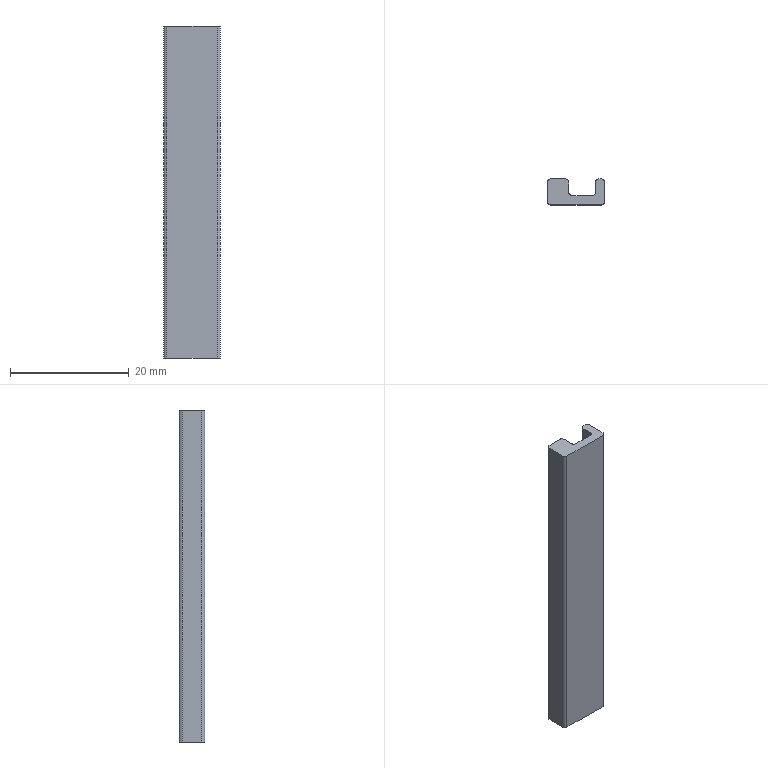Part | NX | features BREP 2 | 2 solids | 36 faces | box 9.6 x 4.3 x 56 mm | volume 3188 mm3 | plane 20 | cylinder 16 | commonest cylinder face diameters 1 x16
STEP:
#1=CARTESIAN_POINT('',(-4.3,2.15,-4.));
#2=VERTEX_POINT('',#1);
#3=CARTESIAN_POINT('',(-4.3,2.15,52.));
#4=VERTEX_POINT('',#3);
#5=CARTESIAN_POINT('',(-4.3,2.15,0.));
#6=DIRECTION('',(0.,0.,1.));
#7=VECTOR('',#6,1000.);
#8=LINE('',#5,#7);
#9=EDGE_CURVE('',#2,#4,#8,.T.);
#10=ORIENTED_EDGE('',*,*,#9,.T.);
#11=CARTESIAN_POINT('',(-1.7,2.15,52.));
#12=VERTEX_POINT('',#11);
#13=CARTESIAN_POINT('',(9.373,2.15,52.));
#14=DIRECTION('',(-1.,0.,0.));
#15=VECTOR('',#14,1000.);
#16=LINE('',#13,#15);
#17=EDGE_CURVE('',#12,#4,#16,.T.);
#18=ORIENTED_EDGE('',*,*,#17,.F.);
#19=CARTESIAN_POINT('',(-1.7,2.15,-4.));
#20=VERTEX_POINT('',#19);
#21=CARTESIAN_POINT('',(-1.7,2.15,0.));
#22=DIRECTION('',(0.,0.,1.));
#23=VECTOR('',#22,1000.);
#24=LINE('',#21,#23);
#25=EDGE_CURVE('',#20,#12,#24,.T.);
#26=ORIENTED_EDGE('',*,*,#25,.F.);
#27=CARTESIAN_POINT('',(9.373,2.15,-4.));
#28=DIRECTION('',(-1.,0.,0.));
#29=VECTOR('',#28,1000.);
#30=LINE('',#27,#29);
#31=EDGE_CURVE('',#20,#2,#30,.T.);
#32=ORIENTED_EDGE('',*,*,#31,.T.);
#33=EDGE_LOOP('',(#10,#18,#26,#32));
#34=FACE_BOUND('',#33,.T.);
#35=CARTESIAN_POINT('',(-1.7,2.15,0.));
#36=DIRECTION('',(0.,1.,0.));
#37=DIRECTION('',(1.,0.,0.));
#38=AXIS2_PLACEMENT_3D('',#35,#36,#37);
#39=PLANE('',#38);
#40=ADVANCED_FACE('',(#34),#39,.T.);
#41=ORIENTED_EDGE('',*,*,#25,.T.);
#42=CARTESIAN_POINT('',(-1.2,1.65,52.));
#43=VERTEX_POINT('',#42);
#44=CARTESIAN_POINT('',(-1.7,1.65,52.));
#45=DIRECTION('',(0.,0.,1.));
#46=DIRECTION('',(1.,0.,0.));
#47=AXIS2_PLACEMENT_3D('',#44,#45,#46);
#48=CIRCLE('',#47,0.5);
#49=EDGE_CURVE('',#43,#12,#48,.T.);
#50=ORIENTED_EDGE('',*,*,#49,.F.);
#51=CARTESIAN_POINT('',(-1.2,1.65,-4.));
#52=VERTEX_POINT('',#51);
#53=CARTESIAN_POINT('',(-1.2,1.65,0.));
#54=DIRECTION('',(0.,0.,1.));
#55=VECTOR('',#54,1000.);
#56=LINE('',#53,#55);
#57=EDGE_CURVE('',#52,#43,#56,.T.);
#58=ORIENTED_EDGE('',*,*,#57,.F.);
#59=CARTESIAN_POINT('',(-1.7,1.65,-4.));
#60=DIRECTION('',(0.,0.,1.));
#61=DIRECTION('',(1.,0.,0.));
#62=AXIS2_PLACEMENT_3D('',#59,#60,#61);
#63=CIRCLE('',#62,0.5);
#64=EDGE_CURVE('',#52,#20,#63,.T.);
#65=ORIENTED_EDGE('',*,*,#64,.T.);
#66=EDGE_LOOP('',(#41,#50,#58,#65));
#67=FACE_BOUND('',#66,.T.);
#68=CARTESIAN_POINT('',(-1.7,1.65,0.));
#69=DIRECTION('',(0.,0.,1.));
#70=DIRECTION('',(-1.,0.,0.));
#71=AXIS2_PLACEMENT_3D('',#68,#69,#70);
#72=CYLINDRICAL_SURFACE('',#71,0.5);
#73=ADVANCED_FACE('',(#67),#72,.T.);
#74=ORIENTED_EDGE('',*,*,#57,.T.);
#75=CARTESIAN_POINT('',(-1.2,-0.15,52.));
#76=VERTEX_POINT('',#75);
#77=CARTESIAN_POINT('',(-1.2,1.628,52.));
#78=DIRECTION('',(0.,1.,0.));
#79=VECTOR('',#78,1000.);
#80=LINE('',#77,#79);
#81=EDGE_CURVE('',#76,#43,#80,.T.);
#82=ORIENTED_EDGE('',*,*,#81,.F.);
#83=CARTESIAN_POINT('',(-1.2,-0.15,-4.));
#84=VERTEX_POINT('',#83);
#85=CARTESIAN_POINT('',(-1.2,-0.15,0.));
#86=DIRECTION('',(0.,0.,1.));
#87=VECTOR('',#86,1000.);
#88=LINE('',#85,#87);
#89=EDGE_CURVE('',#84,#76,#88,.T.);
#90=ORIENTED_EDGE('',*,*,#89,.F.);
#91=CARTESIAN_POINT('',(-1.2,1.628,-4.));
#92=DIRECTION('',(0.,1.,0.));
#93=VECTOR('',#92,1000.);
#94=LINE('',#91,#93);
#95=EDGE_CURVE('',#84,#52,#94,.T.);
#96=ORIENTED_EDGE('',*,*,#95,.T.);
#97=EDGE_LOOP('',(#74,#82,#90,#96));
#98=FACE_BOUND('',#97,.T.);
#99=CARTESIAN_POINT('',(-1.2,-0.15,0.));
#100=DIRECTION('',(1.,0.,0.));
#101=DIRECTION('',(0.,-1.,0.));
#102=AXIS2_PLACEMENT_3D('',#99,#100,#101);
#103=PLANE('',#102);
#104=ADVANCED_FACE('',(#98),#103,.T.);
#105=ORIENTED_EDGE('',*,*,#89,.T.);
#106=CARTESIAN_POINT('',(-0.7,-0.65,52.));
#107=VERTEX_POINT('',#106);
#108=CARTESIAN_POINT('',(-0.7,-0.15,52.));
#109=DIRECTION('',(0.,0.,-1.));
#110=DIRECTION('',(1.,0.,0.));
#111=AXIS2_PLACEMENT_3D('',#108,#109,#110);
#112=CIRCLE('',#111,0.5);
#113=EDGE_CURVE('',#107,#76,#112,.T.);
#114=ORIENTED_EDGE('',*,*,#113,.F.);
#115=CARTESIAN_POINT('',(-0.7,-0.65,-4.));
#116=VERTEX_POINT('',#115);
#117=CARTESIAN_POINT('',(-0.7,-0.65,0.));
#118=DIRECTION('',(0.,0.,1.));
#119=VECTOR('',#118,1000.);
#120=LINE('',#117,#119);
#121=EDGE_CURVE('',#116,#107,#120,.T.);
#122=ORIENTED_EDGE('',*,*,#121,.F.);
#123=CARTESIAN_POINT('',(-0.7,-0.15,-4.));
#124=DIRECTION('',(0.,0.,-1.));
#125=DIRECTION('',(1.,0.,0.));
#126=AXIS2_PLACEMENT_3D('',#123,#124,#125);
#127=CIRCLE('',#126,0.5);
#128=EDGE_CURVE('',#116,#84,#127,.T.);
#129=ORIENTED_EDGE('',*,*,#128,.T.);
#130=EDGE_LOOP('',(#105,#114,#122,#129));
#131=FACE_BOUND('',#130,.T.);
#132=CARTESIAN_POINT('',(-0.7,-0.15,0.));
#133=DIRECTION('',(0.,0.,1.));
#134=DIRECTION('',(-1.,0.,0.));
#135=AXIS2_PLACEMENT_3D('',#132,#133,#134);
#136=CYLINDRICAL_SURFACE('',#135,0.5);
#137=ADVANCED_FACE('',(#131),#136,.F.);
#138=ORIENTED_EDGE('',*,*,#121,.T.);
#139=CARTESIAN_POINT('',(2.8,-0.65,52.));
#140=VERTEX_POINT('',#139);
#141=CARTESIAN_POINT('',(9.373,-0.65,52.));
#142=DIRECTION('',(-1.,0.,0.));
#143=VECTOR('',#142,1000.);
#144=LINE('',#141,#143);
#145=EDGE_CURVE('',#140,#107,#144,.T.);
#146=ORIENTED_EDGE('',*,*,#145,.F.);
#147=CARTESIAN_POINT('',(2.8,-0.65,-4.));
#148=VERTEX_POINT('',#147);
#149=CARTESIAN_POINT('',(2.8,-0.65,0.));
#150=DIRECTION('',(0.,0.,1.));
#151=VECTOR('',#150,1000.);
#152=LINE('',#149,#151);
#153=EDGE_CURVE('',#148,#140,#152,.T.);
#154=ORIENTED_EDGE('',*,*,#153,.F.);
#155=CARTESIAN_POINT('',(9.373,-0.65,-4.));
#156=DIRECTION('',(-1.,0.,0.));
#157=VECTOR('',#156,1000.);
#158=LINE('',#155,#157);
#159=EDGE_CURVE('',#148,#116,#158,.T.);
#160=ORIENTED_EDGE('',*,*,#159,.T.);
#161=EDGE_LOOP('',(#138,#146,#154,#160));
#162=FACE_BOUND('',#161,.T.);
#163=CARTESIAN_POINT('',(2.8,-0.65,0.));
#164=DIRECTION('',(0.,1.,0.));
#165=DIRECTION('',(1.,0.,0.));
#166=AXIS2_PLACEMENT_3D('',#163,#164,#165);
#167=PLANE('',#166);
#168=ADVANCED_FACE('',(#162),#167,.T.);
#169=ORIENTED_EDGE('',*,*,#153,.T.);
#170=CARTESIAN_POINT('',(3.3,-0.15,52.));
#171=VERTEX_POINT('',#170);
#172=CARTESIAN_POINT('',(2.8,-0.15,52.));
#173=DIRECTION('',(0.,0.,-1.));
#174=DIRECTION('',(1.,0.,0.));
#175=AXIS2_PLACEMENT_3D('',#172,#173,#174);
#176=CIRCLE('',#175,0.5);
#177=EDGE_CURVE('',#171,#140,#176,.T.);
#178=ORIENTED_EDGE('',*,*,#177,.F.);
#179=CARTESIAN_POINT('',(3.3,-0.15,-4.));
#180=VERTEX_POINT('',#179);
#181=CARTESIAN_POINT('',(3.3,-0.15,0.));
#182=DIRECTION('',(0.,0.,1.));
#183=VECTOR('',#182,1000.);
#184=LINE('',#181,#183);
#185=EDGE_CURVE('',#180,#171,#184,.T.);
#186=ORIENTED_EDGE('',*,*,#185,.F.);
#187=CARTESIAN_POINT('',(2.8,-0.15,-4.));
#188=DIRECTION('',(0.,0.,-1.));
#189=DIRECTION('',(1.,0.,0.));
#190=AXIS2_PLACEMENT_3D('',#187,#188,#189);
#191=CIRCLE('',#190,0.5);
#192=EDGE_CURVE('',#180,#148,#191,.T.);
#193=ORIENTED_EDGE('',*,*,#192,.T.);
#194=EDGE_LOOP('',(#169,#178,#186,#193));
#195=FACE_BOUND('',#194,.T.);
#196=CARTESIAN_POINT('',(2.8,-0.15,0.));
#197=DIRECTION('',(0.,0.,1.));
#198=DIRECTION('',(-1.,0.,0.));
#199=AXIS2_PLACEMENT_3D('',#196,#197,#198);
#200=CYLINDRICAL_SURFACE('',#199,0.5);
#201=ADVANCED_FACE('',(#195),#200,.F.);
#202=ORIENTED_EDGE('',*,*,#185,.T.);
#203=CARTESIAN_POINT('',(3.3,1.65,52.));
#204=VERTEX_POINT('',#203);
#205=CARTESIAN_POINT('',(3.3,1.628,52.));
#206=DIRECTION('',(0.,-1.,0.));
#207=VECTOR('',#206,1000.);
#208=LINE('',#205,#207);
#209=EDGE_CURVE('',#204,#171,#208,.T.);
#210=ORIENTED_EDGE('',*,*,#209,.F.);
#211=CARTESIAN_POINT('',(3.3,1.65,-4.));
#212=VERTEX_POINT('',#211);
#213=CARTESIAN_POINT('',(3.3,1.65,0.));
#214=DIRECTION('',(0.,0.,1.));
#215=VECTOR('',#214,1000.);
#216=LINE('',#213,#215);
#217=EDGE_CURVE('',#212,#204,#216,.T.);
#218=ORIENTED_EDGE('',*,*,#217,.F.);
#219=CARTESIAN_POINT('',(3.3,1.628,-4.));
#220=DIRECTION('',(0.,-1.,0.));
#221=VECTOR('',#220,1000.);
#222=LINE('',#219,#221);
#223=EDGE_CURVE('',#212,#180,#222,.T.);
#224=ORIENTED_EDGE('',*,*,#223,.T.);
#225=EDGE_LOOP('',(#202,#210,#218,#224));
#226=FACE_BOUND('',#225,.T.);
#227=CARTESIAN_POINT('',(3.3,1.65,0.));
#228=DIRECTION('',(-1.,0.,0.));
#229=DIRECTION('',(0.,1.,0.));
#230=AXIS2_PLACEMENT_3D('',#227,#228,#229);
#231=PLANE('',#230);
#232=ADVANCED_FACE('',(#226),#231,.T.);
#233=ORIENTED_EDGE('',*,*,#217,.T.);
#234=CARTESIAN_POINT('',(3.8,2.15,52.));
#235=VERTEX_POINT('',#234);
#236=CARTESIAN_POINT('',(3.8,1.65,52.));
#237=DIRECTION('',(0.,0.,1.));
#238=DIRECTION('',(1.,0.,0.));
#239=AXIS2_PLACEMENT_3D('',#236,#237,#238);
#240=CIRCLE('',#239,0.5);
#241=EDGE_CURVE('',#235,#204,#240,.T.);
#242=ORIENTED_EDGE('',*,*,#241,.F.);
#243=CARTESIAN_POINT('',(3.8,2.15,-4.));
#244=VERTEX_POINT('',#243);
#245=CARTESIAN_POINT('',(3.8,2.15,0.));
#246=DIRECTION('',(0.,0.,1.));
#247=VECTOR('',#246,1000.);
#248=LINE('',#245,#247);
#249=EDGE_CURVE('',#244,#235,#248,.T.);
#250=ORIENTED_EDGE('',*,*,#249,.F.);
#251=CARTESIAN_POINT('',(3.8,1.65,-4.));
#252=DIRECTION('',(0.,0.,1.));
#253=DIRECTION('',(1.,0.,0.));
#254=AXIS2_PLACEMENT_3D('',#251,#252,#253);
#255=CIRCLE('',#254,0.5);
#256=EDGE_CURVE('',#244,#212,#255,.T.);
#257=ORIENTED_EDGE('',*,*,#256,.T.);
#258=EDGE_LOOP('',(#233,#242,#250,#257));
#259=FACE_BOUND('',#258,.T.);
#260=CARTESIAN_POINT('',(3.8,1.65,0.));
#261=DIRECTION('',(0.,0.,1.));
#262=DIRECTION('',(-1.,0.,0.));
#263=AXIS2_PLACEMENT_3D('',#260,#261,#262);
#264=CYLINDRICAL_SURFACE('',#263,0.5);
#265=ADVANCED_FACE('',(#259),#264,.T.);
#266=ORIENTED_EDGE('',*,*,#249,.T.);
#267=CARTESIAN_POINT('',(4.3,2.15,52.));
#268=VERTEX_POINT('',#267);
#269=CARTESIAN_POINT('',(9.373,2.15,52.));
#270=DIRECTION('',(-1.,0.,0.));
#271=VECTOR('',#270,1000.);
#272=LINE('',#269,#271);
#273=EDGE_CURVE('',#268,#235,#272,.T.);
#274=ORIENTED_EDGE('',*,*,#273,.F.);
#275=CARTESIAN_POINT('',(4.3,2.15,-4.));
#276=VERTEX_POINT('',#275);
#277=CARTESIAN_POINT('',(4.3,2.15,0.));
#278=DIRECTION('',(0.,0.,1.));
#279=VECTOR('',#278,1000.);
#280=LINE('',#277,#279);
#281=EDGE_CURVE('',#276,#268,#280,.T.);
#282=ORIENTED_EDGE('',*,*,#281,.F.);
#283=CARTESIAN_POINT('',(9.373,2.15,-4.));
#284=DIRECTION('',(-1.,0.,0.));
#285=VECTOR('',#284,1000.);
#286=LINE('',#283,#285);
#287=EDGE_CURVE('',#276,#244,#286,.T.);
#288=ORIENTED_EDGE('',*,*,#287,.T.);
#289=EDGE_LOOP('',(#266,#274,#282,#288));
#290=FACE_BOUND('',#289,.T.);
#291=CARTESIAN_POINT('',(4.3,2.15,0.));
#292=DIRECTION('',(0.,1.,0.));
#293=DIRECTION('',(1.,0.,0.));
#294=AXIS2_PLACEMENT_3D('',#291,#292,#293);
#295=PLANE('',#294);
#296=ADVANCED_FACE('',(#290),#295,.T.);
#297=ORIENTED_EDGE('',*,*,#281,.T.);
#298=CARTESIAN_POINT('',(4.8,1.65,52.));
#299=VERTEX_POINT('',#298);
#300=CARTESIAN_POINT('',(4.3,1.65,52.));
#301=DIRECTION('',(0.,0.,1.));
#302=DIRECTION('',(1.,0.,0.));
#303=AXIS2_PLACEMENT_3D('',#300,#301,#302);
#304=CIRCLE('',#303,0.5);
#305=EDGE_CURVE('',#299,#268,#304,.T.);
#306=ORIENTED_EDGE('',*,*,#305,.F.);
#307=CARTESIAN_POINT('',(4.8,1.65,-4.));
#308=VERTEX_POINT('',#307);
#309=CARTESIAN_POINT('',(4.8,1.65,0.));
#310=DIRECTION('',(0.,0.,1.));
#311=VECTOR('',#310,1000.);
#312=LINE('',#309,#311);
#313=EDGE_CURVE('',#308,#299,#312,.T.);
#314=ORIENTED_EDGE('',*,*,#313,.F.);
#315=CARTESIAN_POINT('',(4.3,1.65,-4.));
#316=DIRECTION('',(0.,0.,1.));
#317=DIRECTION('',(1.,0.,0.));
#318=AXIS2_PLACEMENT_3D('',#315,#316,#317);
#319=CIRCLE('',#318,0.5);
#320=EDGE_CURVE('',#308,#276,#319,.T.);
#321=ORIENTED_EDGE('',*,*,#320,.T.);
#322=EDGE_LOOP('',(#297,#306,#314,#321));
#323=FACE_BOUND('',#322,.T.);
#324=CARTESIAN_POINT('',(4.3,1.65,0.));
#325=DIRECTION('',(0.,0.,1.));
#326=DIRECTION('',(-1.,0.,0.));
#327=AXIS2_PLACEMENT_3D('',#324,#325,#326);
#328=CYLINDRICAL_SURFACE('',#327,0.5);
#329=ADVANCED_FACE('',(#323),#328,.T.);
#330=ORIENTED_EDGE('',*,*,#313,.T.);
#331=CARTESIAN_POINT('',(4.8,-1.65,52.));
#332=VERTEX_POINT('',#331);
#333=CARTESIAN_POINT('',(4.8,1.628,52.));
#334=DIRECTION('',(0.,1.,0.));
#335=VECTOR('',#334,1000.);
#336=LINE('',#333,#335);
#337=EDGE_CURVE('',#332,#299,#336,.T.);
#338=ORIENTED_EDGE('',*,*,#337,.F.);
#339=CARTESIAN_POINT('',(4.8,-1.65,-4.));
#340=VERTEX_POINT('',#339);
#341=CARTESIAN_POINT('',(4.8,-1.65,0.));
#342=DIRECTION('',(0.,0.,1.));
#343=VECTOR('',#342,1000.);
#344=LINE('',#341,#343);
#345=EDGE_CURVE('',#340,#332,#344,.T.);
#346=ORIENTED_EDGE('',*,*,#345,.F.);
#347=CARTESIAN_POINT('',(4.8,1.628,-4.));
#348=DIRECTION('',(0.,1.,0.));
#349=VECTOR('',#348,1000.);
#350=LINE('',#347,#349);
#351=EDGE_CURVE('',#340,#308,#350,.T.);
#352=ORIENTED_EDGE('',*,*,#351,.T.);
#353=EDGE_LOOP('',(#330,#338,#346,#352));
#354=FACE_BOUND('',#353,.T.);
#355=CARTESIAN_POINT('',(4.8,-1.65,0.));
#356=DIRECTION('',(1.,0.,0.));
#357=DIRECTION('',(0.,-1.,0.));
#358=AXIS2_PLACEMENT_3D('',#355,#356,#357);
#359=PLANE('',#358);
#360=ADVANCED_FACE('',(#354),#359,.T.);
#361=ORIENTED_EDGE('',*,*,#345,.T.);
#362=CARTESIAN_POINT('',(4.3,-2.15,52.));
#363=VERTEX_POINT('',#362);
#364=CARTESIAN_POINT('',(4.3,-1.65,52.));
#365=DIRECTION('',(0.,0.,1.));
#366=DIRECTION('',(1.,0.,0.));
#367=AXIS2_PLACEMENT_3D('',#364,#365,#366);
#368=CIRCLE('',#367,0.5);
#369=EDGE_CURVE('',#363,#332,#368,.T.);
#370=ORIENTED_EDGE('',*,*,#369,.F.);
#371=CARTESIAN_POINT('',(4.3,-2.15,-4.));
#372=VERTEX_POINT('',#371);
#373=CARTESIAN_POINT('',(4.3,-2.15,0.));
#374=DIRECTION('',(0.,0.,1.));
#375=VECTOR('',#374,1000.);
#376=LINE('',#373,#375);
#377=EDGE_CURVE('',#372,#363,#376,.T.);
#378=ORIENTED_EDGE('',*,*,#377,.F.);
#379=CARTESIAN_POINT('',(4.3,-1.65,-4.));
#380=DIRECTION('',(0.,0.,1.));
#381=DIRECTION('',(1.,0.,0.));
#382=AXIS2_PLACEMENT_3D('',#379,#380,#381);
#383=CIRCLE('',#382,0.5);
#384=EDGE_CURVE('',#372,#340,#383,.T.);
#385=ORIENTED_EDGE('',*,*,#384,.T.);
#386=EDGE_LOOP('',(#361,#370,#378,#385));
#387=FACE_BOUND('',#386,.T.);
#388=CARTESIAN_POINT('',(4.3,-1.65,0.));
#389=DIRECTION('',(0.,0.,1.));
#390=DIRECTION('',(-1.,0.,0.));
#391=AXIS2_PLACEMENT_3D('',#388,#389,#390);
#392=CYLINDRICAL_SURFACE('',#391,0.5);
#393=ADVANCED_FACE('',(#387),#392,.T.);
#394=ORIENTED_EDGE('',*,*,#377,.T.);
#395=CARTESIAN_POINT('',(-4.3,-2.15,52.));
#396=VERTEX_POINT('',#395);
#397=CARTESIAN_POINT('',(9.373,-2.15,52.));
#398=DIRECTION('',(1.,0.,0.));
#399=VECTOR('',#398,1000.);
#400=LINE('',#397,#399);
#401=EDGE_CURVE('',#396,#363,#400,.T.);
#402=ORIENTED_EDGE('',*,*,#401,.F.);
#403=CARTESIAN_POINT('',(-4.3,-2.15,-4.));
#404=VERTEX_POINT('',#403);
#405=CARTESIAN_POINT('',(-4.3,-2.15,0.));
#406=DIRECTION('',(0.,0.,1.));
#407=VECTOR('',#406,1000.);
#408=LINE('',#405,#407);
#409=EDGE_CURVE('',#404,#396,#408,.T.);
#410=ORIENTED_EDGE('',*,*,#409,.F.);
#411=CARTESIAN_POINT('',(9.373,-2.15,-4.));
#412=DIRECTION('',(1.,0.,0.));
#413=VECTOR('',#412,1000.);
#414=LINE('',#411,#413);
#415=EDGE_CURVE('',#404,#372,#414,.T.);
#416=ORIENTED_EDGE('',*,*,#415,.T.);
#417=EDGE_LOOP('',(#394,#402,#410,#416));
#418=FACE_BOUND('',#417,.T.);
#419=CARTESIAN_POINT('',(-4.3,-2.15,0.));
#420=DIRECTION('',(0.,-1.,0.));
#421=DIRECTION('',(-1.,0.,0.));
#422=AXIS2_PLACEMENT_3D('',#419,#420,#421);
#423=PLANE('',#422);
#424=ADVANCED_FACE('',(#418),#423,.T.);
#425=ORIENTED_EDGE('',*,*,#409,.T.);
#426=CARTESIAN_POINT('',(-4.8,-1.65,52.));
#427=VERTEX_POINT('',#426);
#428=CARTESIAN_POINT('',(-4.3,-1.65,52.));
#429=DIRECTION('',(0.,0.,1.));
#430=DIRECTION('',(1.,0.,0.));
#431=AXIS2_PLACEMENT_3D('',#428,#429,#430);
#432=CIRCLE('',#431,0.5);
#433=EDGE_CURVE('',#427,#396,#432,.T.);
#434=ORIENTED_EDGE('',*,*,#433,.F.);
#435=CARTESIAN_POINT('',(-4.8,-1.65,-4.));
#436=VERTEX_POINT('',#435);
#437=CARTESIAN_POINT('',(-4.8,-1.65,0.));
#438=DIRECTION('',(0.,0.,1.));
#439=VECTOR('',#438,1000.);
#440=LINE('',#437,#439);
#441=EDGE_CURVE('',#436,#427,#440,.T.);
#442=ORIENTED_EDGE('',*,*,#441,.F.);
#443=CARTESIAN_POINT('',(-4.3,-1.65,-4.));
#444=DIRECTION('',(0.,0.,1.));
#445=DIRECTION('',(1.,0.,0.));
#446=AXIS2_PLACEMENT_3D('',#443,#444,#445);
#447=CIRCLE('',#446,0.5);
#448=EDGE_CURVE('',#436,#404,#447,.T.);
#449=ORIENTED_EDGE('',*,*,#448,.T.);
#450=EDGE_LOOP('',(#425,#434,#442,#449));
#451=FACE_BOUND('',#450,.T.);
#452=CARTESIAN_POINT('',(-4.3,-1.65,0.));
#453=DIRECTION('',(0.,0.,1.));
#454=DIRECTION('',(-1.,0.,0.));
#455=AXIS2_PLACEMENT_3D('',#452,#453,#454);
#456=CYLINDRICAL_SURFACE('',#455,0.5);
#457=ADVANCED_FACE('',(#451),#456,.T.);
#458=ORIENTED_EDGE('',*,*,#441,.T.);
#459=CARTESIAN_POINT('',(-4.8,1.65,52.));
#460=VERTEX_POINT('',#459);
#461=CARTESIAN_POINT('',(-4.8,1.628,52.));
#462=DIRECTION('',(0.,-1.,0.));
#463=VECTOR('',#462,1000.);
#464=LINE('',#461,#463);
#465=EDGE_CURVE('',#460,#427,#464,.T.);
#466=ORIENTED_EDGE('',*,*,#465,.F.);
#467=CARTESIAN_POINT('',(-4.8,1.65,-4.));
#468=VERTEX_POINT('',#467);
#469=CARTESIAN_POINT('',(-4.8,1.65,0.));
#470=DIRECTION('',(0.,0.,1.));
#471=VECTOR('',#470,1000.);
#472=LINE('',#469,#471);
#473=EDGE_CURVE('',#468,#460,#472,.T.);
#474=ORIENTED_EDGE('',*,*,#473,.F.);
#475=CARTESIAN_POINT('',(-4.8,1.628,-4.));
#476=DIRECTION('',(0.,-1.,0.));
#477=VECTOR('',#476,1000.);
#478=LINE('',#475,#477);
#479=EDGE_CURVE('',#468,#436,#478,.T.);
#480=ORIENTED_EDGE('',*,*,#479,.T.);
#481=EDGE_LOOP('',(#458,#466,#474,#480));
#482=FACE_BOUND('',#481,.T.);
#483=CARTESIAN_POINT('',(-4.8,1.65,0.));
#484=DIRECTION('',(-1.,0.,0.));
#485=DIRECTION('',(0.,1.,0.));
#486=AXIS2_PLACEMENT_3D('',#483,#484,#485);
#487=PLANE('',#486);
#488=ADVANCED_FACE('',(#482),#487,.T.);
#489=CARTESIAN_POINT('',(-4.3,1.65,-4.));
#490=DIRECTION('',(0.,0.,1.));
#491=DIRECTION('',(1.,0.,0.));
#492=AXIS2_PLACEMENT_3D('',#489,#490,#491);
#493=CIRCLE('',#492,0.5);
#494=EDGE_CURVE('',#2,#468,#493,.T.);
#495=ORIENTED_EDGE('',*,*,#494,.T.);
#496=ORIENTED_EDGE('',*,*,#473,.T.);
#497=CARTESIAN_POINT('',(-4.3,1.65,52.));
#498=DIRECTION('',(0.,0.,1.));
#499=DIRECTION('',(1.,0.,0.));
#500=AXIS2_PLACEMENT_3D('',#497,#498,#499);
#501=CIRCLE('',#500,0.5);
#502=EDGE_CURVE('',#4,#460,#501,.T.);
#503=ORIENTED_EDGE('',*,*,#502,.F.);
#504=ORIENTED_EDGE('',*,*,#9,.F.);
#505=EDGE_LOOP('',(#495,#496,#503,#504));
#506=FACE_BOUND('',#505,.T.);
#507=CARTESIAN_POINT('',(-4.3,1.65,0.));
#508=DIRECTION('',(0.,0.,1.));
#509=DIRECTION('',(-1.,0.,0.));
#510=AXIS2_PLACEMENT_3D('',#507,#508,#509);
#511=CYLINDRICAL_SURFACE('',#510,0.5);
#512=ADVANCED_FACE('',(#506),#511,.T.);
#513=ORIENTED_EDGE('',*,*,#465,.T.);
#514=ORIENTED_EDGE('',*,*,#433,.T.);
#515=ORIENTED_EDGE('',*,*,#401,.T.);
#516=ORIENTED_EDGE('',*,*,#369,.T.);
#517=ORIENTED_EDGE('',*,*,#337,.T.);
#518=ORIENTED_EDGE('',*,*,#305,.T.);
#519=ORIENTED_EDGE('',*,*,#273,.T.);
#520=ORIENTED_EDGE('',*,*,#241,.T.);
#521=ORIENTED_EDGE('',*,*,#209,.T.);
#522=ORIENTED_EDGE('',*,*,#177,.T.);
#523=ORIENTED_EDGE('',*,*,#145,.T.);
#524=ORIENTED_EDGE('',*,*,#113,.T.);
#525=ORIENTED_EDGE('',*,*,#81,.T.);
#526=ORIENTED_EDGE('',*,*,#49,.T.);
#527=ORIENTED_EDGE('',*,*,#17,.T.);
#528=ORIENTED_EDGE('',*,*,#502,.T.);
#529=EDGE_LOOP('',(#513,#514,#515,#516,#517,#518,#519,#520,#521,#522,#523,#524,#525,#526,#527,#528));
#530=FACE_BOUND('',#529,.T.);
#531=CARTESIAN_POINT('',(9.373,1.628,52.));
#532=DIRECTION('',(0.,0.,1.));
#533=DIRECTION('',(-1.,0.,0.));
#534=AXIS2_PLACEMENT_3D('',#531,#532,#533);
#535=PLANE('',#534);
#536=ADVANCED_FACE('',(#530),#535,.T.);
#537=ORIENTED_EDGE('',*,*,#479,.F.);
#538=ORIENTED_EDGE('',*,*,#494,.F.);
#539=ORIENTED_EDGE('',*,*,#31,.F.);
#540=ORIENTED_EDGE('',*,*,#64,.F.);
#541=ORIENTED_EDGE('',*,*,#95,.F.);
#542=ORIENTED_EDGE('',*,*,#128,.F.);
#543=ORIENTED_EDGE('',*,*,#159,.F.);
#544=ORIENTED_EDGE('',*,*,#192,.F.);
#545=ORIENTED_EDGE('',*,*,#223,.F.);
#546=ORIENTED_EDGE('',*,*,#256,.F.);
#547=ORIENTED_EDGE('',*,*,#287,.F.);
#548=ORIENTED_EDGE('',*,*,#320,.F.);
#549=ORIENTED_EDGE('',*,*,#351,.F.);
#550=ORIENTED_EDGE('',*,*,#384,.F.);
#551=ORIENTED_EDGE('',*,*,#415,.F.);
#552=ORIENTED_EDGE('',*,*,#448,.F.);
#553=EDGE_LOOP('',(#537,#538,#539,#540,#541,#542,#543,#544,#545,#546,#547,#548,#549,#550,#551,#552));
#554=FACE_BOUND('',#553,.T.);
#555=CARTESIAN_POINT('',(9.373,1.628,-4.));
#556=DIRECTION('',(0.,0.,1.));
#557=DIRECTION('',(-1.,0.,0.));
#558=AXIS2_PLACEMENT_3D('',#555,#556,#557);
#559=PLANE('',#558);
#560=ADVANCED_FACE('',(#554),#559,.F.);
#561=CLOSED_SHELL('',(#40,#73,#104,#137,#168,#201,#232,#265,#296,#329,#360,#393,#424,#457,#488,#512,#536,#560));
#562=MANIFOLD_SOLID_BREP('',#561);
#563=CARTESIAN_POINT('',(-4.3,2.15,-4.));
#564=VERTEX_POINT('',#563);
#565=CARTESIAN_POINT('',(-4.3,2.15,52.));
#566=VERTEX_POINT('',#565);
#567=CARTESIAN_POINT('',(-4.3,2.15,0.));
#568=DIRECTION('',(0.,0.,1.));
#569=VECTOR('',#568,1000.);
#570=LINE('',#567,#569);
#571=EDGE_CURVE('',#564,#566,#570,.T.);
#572=ORIENTED_EDGE('',*,*,#571,.T.);
#573=CARTESIAN_POINT('',(-1.7,2.15,52.));
#574=VERTEX_POINT('',#573);
#575=CARTESIAN_POINT('',(9.373,2.15,52.));
#576=DIRECTION('',(-1.,0.,0.));
#577=VECTOR('',#576,1000.);
#578=LINE('',#575,#577);
#579=EDGE_CURVE('',#574,#566,#578,.T.);
#580=ORIENTED_EDGE('',*,*,#579,.F.);
#581=CARTESIAN_POINT('',(-1.7,2.15,-4.));
#582=VERTEX_POINT('',#581);
#583=CARTESIAN_POINT('',(-1.7,2.15,0.));
#584=DIRECTION('',(0.,0.,1.));
#585=VECTOR('',#584,1000.);
#586=LINE('',#583,#585);
#587=EDGE_CURVE('',#582,#574,#586,.T.);
#588=ORIENTED_EDGE('',*,*,#587,.F.);
#589=CARTESIAN_POINT('',(9.373,2.15,-4.));
#590=DIRECTION('',(-1.,0.,0.));
#591=VECTOR('',#590,1000.);
#592=LINE('',#589,#591);
#593=EDGE_CURVE('',#582,#564,#592,.T.);
#594=ORIENTED_EDGE('',*,*,#593,.T.);
#595=EDGE_LOOP('',(#572,#580,#588,#594));
#596=FACE_BOUND('',#595,.T.);
#597=CARTESIAN_POINT('',(-1.7,2.15,0.));
#598=DIRECTION('',(0.,1.,0.));
#599=DIRECTION('',(1.,0.,0.));
#600=AXIS2_PLACEMENT_3D('',#597,#598,#599);
#601=PLANE('',#600);
#602=ADVANCED_FACE('',(#596),#601,.T.);
#603=ORIENTED_EDGE('',*,*,#587,.T.);
#604=CARTESIAN_POINT('',(-1.2,1.65,52.));
#605=VERTEX_POINT('',#604);
#606=CARTESIAN_POINT('',(-1.7,1.65,52.));
#607=DIRECTION('',(0.,0.,1.));
#608=DIRECTION('',(1.,0.,0.));
#609=AXIS2_PLACEMENT_3D('',#606,#607,#608);
#610=CIRCLE('',#609,0.5);
#611=EDGE_CURVE('',#605,#574,#610,.T.);
#612=ORIENTED_EDGE('',*,*,#611,.F.);
#613=CARTESIAN_POINT('',(-1.2,1.65,-4.));
#614=VERTEX_POINT('',#613);
#615=CARTESIAN_POINT('',(-1.2,1.65,0.));
#616=DIRECTION('',(0.,0.,1.));
#617=VECTOR('',#616,1000.);
#618=LINE('',#615,#617);
#619=EDGE_CURVE('',#614,#605,#618,.T.);
#620=ORIENTED_EDGE('',*,*,#619,.F.);
#621=CARTESIAN_POINT('',(-1.7,1.65,-4.));
#622=DIRECTION('',(0.,0.,1.));
#623=DIRECTION('',(1.,0.,0.));
#624=AXIS2_PLACEMENT_3D('',#621,#622,#623);
#625=CIRCLE('',#624,0.5);
#626=EDGE_CURVE('',#614,#582,#625,.T.);
#627=ORIENTED_EDGE('',*,*,#626,.T.);
#628=EDGE_LOOP('',(#603,#612,#620,#627));
#629=FACE_BOUND('',#628,.T.);
#630=CARTESIAN_POINT('',(-1.7,1.65,0.));
#631=DIRECTION('',(0.,0.,1.));
#632=DIRECTION('',(-1.,0.,0.));
#633=AXIS2_PLACEMENT_3D('',#630,#631,#632);
#634=CYLINDRICAL_SURFACE('',#633,0.5);
#635=ADVANCED_FACE('',(#629),#634,.T.);
#636=ORIENTED_EDGE('',*,*,#619,.T.);
#637=CARTESIAN_POINT('',(-1.2,-0.15,52.));
#638=VERTEX_POINT('',#637);
#639=CARTESIAN_POINT('',(-1.2,1.628,52.));
#640=DIRECTION('',(0.,1.,0.));
#641=VECTOR('',#640,1000.);
#642=LINE('',#639,#641);
#643=EDGE_CURVE('',#638,#605,#642,.T.);
#644=ORIENTED_EDGE('',*,*,#643,.F.);
#645=CARTESIAN_POINT('',(-1.2,-0.15,-4.));
#646=VERTEX_POINT('',#645);
#647=CARTESIAN_POINT('',(-1.2,-0.15,0.));
#648=DIRECTION('',(0.,0.,1.));
#649=VECTOR('',#648,1000.);
#650=LINE('',#647,#649);
#651=EDGE_CURVE('',#646,#638,#650,.T.);
#652=ORIENTED_EDGE('',*,*,#651,.F.);
#653=CARTESIAN_POINT('',(-1.2,1.628,-4.));
#654=DIRECTION('',(0.,1.,0.));
#655=VECTOR('',#654,1000.);
#656=LINE('',#653,#655);
#657=EDGE_CURVE('',#646,#614,#656,.T.);
#658=ORIENTED_EDGE('',*,*,#657,.T.);
#659=EDGE_LOOP('',(#636,#644,#652,#658));
#660=FACE_BOUND('',#659,.T.);
#661=CARTESIAN_POINT('',(-1.2,-0.15,0.));
#662=DIRECTION('',(1.,0.,0.));
#663=DIRECTION('',(0.,-1.,0.));
#664=AXIS2_PLACEMENT_3D('',#661,#662,#663);
#665=PLANE('',#664);
#666=ADVANCED_FACE('',(#660),#665,.T.);
#667=ORIENTED_EDGE('',*,*,#651,.T.);
#668=CARTESIAN_POINT('',(-0.7,-0.65,52.));
#669=VERTEX_POINT('',#668);
#670=CARTESIAN_POINT('',(-0.7,-0.15,52.));
#671=DIRECTION('',(0.,0.,-1.));
#672=DIRECTION('',(1.,0.,0.));
#673=AXIS2_PLACEMENT_3D('',#670,#671,#672);
#674=CIRCLE('',#673,0.5);
#675=EDGE_CURVE('',#669,#638,#674,.T.);
#676=ORIENTED_EDGE('',*,*,#675,.F.);
#677=CARTESIAN_POINT('',(-0.7,-0.65,-4.));
#678=VERTEX_POINT('',#677);
#679=CARTESIAN_POINT('',(-0.7,-0.65,0.));
#680=DIRECTION('',(0.,0.,1.));
#681=VECTOR('',#680,1000.);
#682=LINE('',#679,#681);
#683=EDGE_CURVE('',#678,#669,#682,.T.);
#684=ORIENTED_EDGE('',*,*,#683,.F.);
#685=CARTESIAN_POINT('',(-0.7,-0.15,-4.));
#686=DIRECTION('',(0.,0.,-1.));
#687=DIRECTION('',(1.,0.,0.));
#688=AXIS2_PLACEMENT_3D('',#685,#686,#687);
#689=CIRCLE('',#688,0.5);
#690=EDGE_CURVE('',#678,#646,#689,.T.);
#691=ORIENTED_EDGE('',*,*,#690,.T.);
#692=EDGE_LOOP('',(#667,#676,#684,#691));
#693=FACE_BOUND('',#692,.T.);
#694=CARTESIAN_POINT('',(-0.7,-0.15,0.));
#695=DIRECTION('',(0.,0.,1.));
#696=DIRECTION('',(-1.,0.,0.));
#697=AXIS2_PLACEMENT_3D('',#694,#695,#696);
#698=CYLINDRICAL_SURFACE('',#697,0.5);
#699=ADVANCED_FACE('',(#693),#698,.F.);
#700=ORIENTED_EDGE('',*,*,#683,.T.);
#701=CARTESIAN_POINT('',(2.8,-0.65,52.));
#702=VERTEX_POINT('',#701);
#703=CARTESIAN_POINT('',(9.373,-0.65,52.));
#704=DIRECTION('',(-1.,0.,0.));
#705=VECTOR('',#704,1000.);
#706=LINE('',#703,#705);
#707=EDGE_CURVE('',#702,#669,#706,.T.);
#708=ORIENTED_EDGE('',*,*,#707,.F.);
#709=CARTESIAN_POINT('',(2.8,-0.65,-4.));
#710=VERTEX_POINT('',#709);
#711=CARTESIAN_POINT('',(2.8,-0.65,0.));
#712=DIRECTION('',(0.,0.,1.));
#713=VECTOR('',#712,1000.);
#714=LINE('',#711,#713);
#715=EDGE_CURVE('',#710,#702,#714,.T.);
#716=ORIENTED_EDGE('',*,*,#715,.F.);
#717=CARTESIAN_POINT('',(9.373,-0.65,-4.));
#718=DIRECTION('',(-1.,0.,0.));
#719=VECTOR('',#718,1000.);
#720=LINE('',#717,#719);
#721=EDGE_CURVE('',#710,#678,#720,.T.);
#722=ORIENTED_EDGE('',*,*,#721,.T.);
#723=EDGE_LOOP('',(#700,#708,#716,#722));
#724=FACE_BOUND('',#723,.T.);
#725=CARTESIAN_POINT('',(2.8,-0.65,0.));
#726=DIRECTION('',(0.,1.,0.));
#727=DIRECTION('',(1.,0.,0.));
#728=AXIS2_PLACEMENT_3D('',#725,#726,#727);
#729=PLANE('',#728);
#730=ADVANCED_FACE('',(#724),#729,.T.);
#731=ORIENTED_EDGE('',*,*,#715,.T.);
#732=CARTESIAN_POINT('',(3.3,-0.15,52.));
#733=VERTEX_POINT('',#732);
#734=CARTESIAN_POINT('',(2.8,-0.15,52.));
#735=DIRECTION('',(0.,0.,-1.));
#736=DIRECTION('',(1.,0.,0.));
#737=AXIS2_PLACEMENT_3D('',#734,#735,#736);
#738=CIRCLE('',#737,0.5);
#739=EDGE_CURVE('',#733,#702,#738,.T.);
#740=ORIENTED_EDGE('',*,*,#739,.F.);
#741=CARTESIAN_POINT('',(3.3,-0.15,-4.));
#742=VERTEX_POINT('',#741);
#743=CARTESIAN_POINT('',(3.3,-0.15,0.));
#744=DIRECTION('',(0.,0.,1.));
#745=VECTOR('',#744,1000.);
#746=LINE('',#743,#745);
#747=EDGE_CURVE('',#742,#733,#746,.T.);
#748=ORIENTED_EDGE('',*,*,#747,.F.);
#749=CARTESIAN_POINT('',(2.8,-0.15,-4.));
#750=DIRECTION('',(0.,0.,-1.));
#751=DIRECTION('',(1.,0.,0.));
#752=AXIS2_PLACEMENT_3D('',#749,#750,#751);
#753=CIRCLE('',#752,0.5);
#754=EDGE_CURVE('',#742,#710,#753,.T.);
#755=ORIENTED_EDGE('',*,*,#754,.T.);
#756=EDGE_LOOP('',(#731,#740,#748,#755));
#757=FACE_BOUND('',#756,.T.);
#758=CARTESIAN_POINT('',(2.8,-0.15,0.));
#759=DIRECTION('',(0.,0.,1.));
#760=DIRECTION('',(-1.,0.,0.));
#761=AXIS2_PLACEMENT_3D('',#758,#759,#760);
#762=CYLINDRICAL_SURFACE('',#761,0.5);
#763=ADVANCED_FACE('',(#757),#762,.F.);
#764=ORIENTED_EDGE('',*,*,#747,.T.);
#765=CARTESIAN_POINT('',(3.3,1.65,52.));
#766=VERTEX_POINT('',#765);
#767=CARTESIAN_POINT('',(3.3,1.628,52.));
#768=DIRECTION('',(0.,-1.,0.));
#769=VECTOR('',#768,1000.);
#770=LINE('',#767,#769);
#771=EDGE_CURVE('',#766,#733,#770,.T.);
#772=ORIENTED_EDGE('',*,*,#771,.F.);
#773=CARTESIAN_POINT('',(3.3,1.65,-4.));
#774=VERTEX_POINT('',#773);
#775=CARTESIAN_POINT('',(3.3,1.65,0.));
#776=DIRECTION('',(0.,0.,1.));
#777=VECTOR('',#776,1000.);
#778=LINE('',#775,#777);
#779=EDGE_CURVE('',#774,#766,#778,.T.);
#780=ORIENTED_EDGE('',*,*,#779,.F.);
#781=CARTESIAN_POINT('',(3.3,1.628,-4.));
#782=DIRECTION('',(0.,-1.,0.));
#783=VECTOR('',#782,1000.);
#784=LINE('',#781,#783);
#785=EDGE_CURVE('',#774,#742,#784,.T.);
#786=ORIENTED_EDGE('',*,*,#785,.T.);
#787=EDGE_LOOP('',(#764,#772,#780,#786));
#788=FACE_BOUND('',#787,.T.);
#789=CARTESIAN_POINT('',(3.3,1.65,0.));
#790=DIRECTION('',(-1.,0.,0.));
#791=DIRECTION('',(0.,1.,0.));
#792=AXIS2_PLACEMENT_3D('',#789,#790,#791);
#793=PLANE('',#792);
#794=ADVANCED_FACE('',(#788),#793,.T.);
#795=ORIENTED_EDGE('',*,*,#779,.T.);
#796=CARTESIAN_POINT('',(3.8,2.15,52.));
#797=VERTEX_POINT('',#796);
#798=CARTESIAN_POINT('',(3.8,1.65,52.));
#799=DIRECTION('',(0.,0.,1.));
#800=DIRECTION('',(1.,0.,0.));
#801=AXIS2_PLACEMENT_3D('',#798,#799,#800);
#802=CIRCLE('',#801,0.5);
#803=EDGE_CURVE('',#797,#766,#802,.T.);
#804=ORIENTED_EDGE('',*,*,#803,.F.);
#805=CARTESIAN_POINT('',(3.8,2.15,-4.));
#806=VERTEX_POINT('',#805);
#807=CARTESIAN_POINT('',(3.8,2.15,0.));
#808=DIRECTION('',(0.,0.,1.));
#809=VECTOR('',#808,1000.);
#810=LINE('',#807,#809);
#811=EDGE_CURVE('',#806,#797,#810,.T.);
#812=ORIENTED_EDGE('',*,*,#811,.F.);
#813=CARTESIAN_POINT('',(3.8,1.65,-4.));
#814=DIRECTION('',(0.,0.,1.));
#815=DIRECTION('',(1.,0.,0.));
#816=AXIS2_PLACEMENT_3D('',#813,#814,#815);
#817=CIRCLE('',#816,0.5);
#818=EDGE_CURVE('',#806,#774,#817,.T.);
#819=ORIENTED_EDGE('',*,*,#818,.T.);
#820=EDGE_LOOP('',(#795,#804,#812,#819));
#821=FACE_BOUND('',#820,.T.);
#822=CARTESIAN_POINT('',(3.8,1.65,0.));
#823=DIRECTION('',(0.,0.,1.));
#824=DIRECTION('',(-1.,0.,0.));
#825=AXIS2_PLACEMENT_3D('',#822,#823,#824);
#826=CYLINDRICAL_SURFACE('',#825,0.5);
#827=ADVANCED_FACE('',(#821),#826,.T.);
#828=ORIENTED_EDGE('',*,*,#811,.T.);
#829=CARTESIAN_POINT('',(4.3,2.15,52.));
#830=VERTEX_POINT('',#829);
#831=CARTESIAN_POINT('',(9.373,2.15,52.));
#832=DIRECTION('',(-1.,0.,0.));
#833=VECTOR('',#832,1000.);
#834=LINE('',#831,#833);
#835=EDGE_CURVE('',#830,#797,#834,.T.);
#836=ORIENTED_EDGE('',*,*,#835,.F.);
#837=CARTESIAN_POINT('',(4.3,2.15,-4.));
#838=VERTEX_POINT('',#837);
#839=CARTESIAN_POINT('',(4.3,2.15,0.));
#840=DIRECTION('',(0.,0.,1.));
#841=VECTOR('',#840,1000.);
#842=LINE('',#839,#841);
#843=EDGE_CURVE('',#838,#830,#842,.T.);
#844=ORIENTED_EDGE('',*,*,#843,.F.);
#845=CARTESIAN_POINT('',(9.373,2.15,-4.));
#846=DIRECTION('',(-1.,0.,0.));
#847=VECTOR('',#846,1000.);
#848=LINE('',#845,#847);
#849=EDGE_CURVE('',#838,#806,#848,.T.);
#850=ORIENTED_EDGE('',*,*,#849,.T.);
#851=EDGE_LOOP('',(#828,#836,#844,#850));
#852=FACE_BOUND('',#851,.T.);
#853=CARTESIAN_POINT('',(4.3,2.15,0.));
#854=DIRECTION('',(0.,1.,0.));
#855=DIRECTION('',(1.,0.,0.));
#856=AXIS2_PLACEMENT_3D('',#853,#854,#855);
#857=PLANE('',#856);
#858=ADVANCED_FACE('',(#852),#857,.T.);
#859=ORIENTED_EDGE('',*,*,#843,.T.);
#860=CARTESIAN_POINT('',(4.8,1.65,52.));
#861=VERTEX_POINT('',#860);
#862=CARTESIAN_POINT('',(4.3,1.65,52.));
#863=DIRECTION('',(0.,0.,1.));
#864=DIRECTION('',(1.,0.,0.));
#865=AXIS2_PLACEMENT_3D('',#862,#863,#864);
#866=CIRCLE('',#865,0.5);
#867=EDGE_CURVE('',#861,#830,#866,.T.);
#868=ORIENTED_EDGE('',*,*,#867,.F.);
#869=CARTESIAN_POINT('',(4.8,1.65,-4.));
#870=VERTEX_POINT('',#869);
#871=CARTESIAN_POINT('',(4.8,1.65,0.));
#872=DIRECTION('',(0.,0.,1.));
#873=VECTOR('',#872,1000.);
#874=LINE('',#871,#873);
#875=EDGE_CURVE('',#870,#861,#874,.T.);
#876=ORIENTED_EDGE('',*,*,#875,.F.);
#877=CARTESIAN_POINT('',(4.3,1.65,-4.));
#878=DIRECTION('',(0.,0.,1.));
#879=DIRECTION('',(1.,0.,0.));
#880=AXIS2_PLACEMENT_3D('',#877,#878,#879);
#881=CIRCLE('',#880,0.5);
#882=EDGE_CURVE('',#870,#838,#881,.T.);
#883=ORIENTED_EDGE('',*,*,#882,.T.);
#884=EDGE_LOOP('',(#859,#868,#876,#883));
#885=FACE_BOUND('',#884,.T.);
#886=CARTESIAN_POINT('',(4.3,1.65,0.));
#887=DIRECTION('',(0.,0.,1.));
#888=DIRECTION('',(-1.,0.,0.));
#889=AXIS2_PLACEMENT_3D('',#886,#887,#888);
#890=CYLINDRICAL_SURFACE('',#889,0.5);
#891=ADVANCED_FACE('',(#885),#890,.T.);
#892=ORIENTED_EDGE('',*,*,#875,.T.);
#893=CARTESIAN_POINT('',(4.8,-1.65,52.));
#894=VERTEX_POINT('',#893);
#895=CARTESIAN_POINT('',(4.8,1.628,52.));
#896=DIRECTION('',(0.,1.,0.));
#897=VECTOR('',#896,1000.);
#898=LINE('',#895,#897);
#899=EDGE_CURVE('',#894,#861,#898,.T.);
#900=ORIENTED_EDGE('',*,*,#899,.F.);
#901=CARTESIAN_POINT('',(4.8,-1.65,-4.));
#902=VERTEX_POINT('',#901);
#903=CARTESIAN_POINT('',(4.8,-1.65,0.));
#904=DIRECTION('',(0.,0.,1.));
#905=VECTOR('',#904,1000.);
#906=LINE('',#903,#905);
#907=EDGE_CURVE('',#902,#894,#906,.T.);
#908=ORIENTED_EDGE('',*,*,#907,.F.);
#909=CARTESIAN_POINT('',(4.8,1.628,-4.));
#910=DIRECTION('',(0.,1.,0.));
#911=VECTOR('',#910,1000.);
#912=LINE('',#909,#911);
#913=EDGE_CURVE('',#902,#870,#912,.T.);
#914=ORIENTED_EDGE('',*,*,#913,.T.);
#915=EDGE_LOOP('',(#892,#900,#908,#914));
#916=FACE_BOUND('',#915,.T.);
#917=CARTESIAN_POINT('',(4.8,-1.65,0.));
#918=DIRECTION('',(1.,0.,0.));
#919=DIRECTION('',(0.,-1.,0.));
#920=AXIS2_PLACEMENT_3D('',#917,#918,#919);
#921=PLANE('',#920);
#922=ADVANCED_FACE('',(#916),#921,.T.);
#923=ORIENTED_EDGE('',*,*,#907,.T.);
#924=CARTESIAN_POINT('',(4.3,-2.15,52.));
#925=VERTEX_POINT('',#924);
#926=CARTESIAN_POINT('',(4.3,-1.65,52.));
#927=DIRECTION('',(0.,0.,1.));
#928=DIRECTION('',(1.,0.,0.));
#929=AXIS2_PLACEMENT_3D('',#926,#927,#928);
#930=CIRCLE('',#929,0.5);
#931=EDGE_CURVE('',#925,#894,#930,.T.);
#932=ORIENTED_EDGE('',*,*,#931,.F.);
#933=CARTESIAN_POINT('',(4.3,-2.15,-4.));
#934=VERTEX_POINT('',#933);
#935=CARTESIAN_POINT('',(4.3,-2.15,0.));
#936=DIRECTION('',(0.,0.,1.));
#937=VECTOR('',#936,1000.);
#938=LINE('',#935,#937);
#939=EDGE_CURVE('',#934,#925,#938,.T.);
#940=ORIENTED_EDGE('',*,*,#939,.F.);
#941=CARTESIAN_POINT('',(4.3,-1.65,-4.));
#942=DIRECTION('',(0.,0.,1.));
#943=DIRECTION('',(1.,0.,0.));
#944=AXIS2_PLACEMENT_3D('',#941,#942,#943);
#945=CIRCLE('',#944,0.5);
#946=EDGE_CURVE('',#934,#902,#945,.T.);
#947=ORIENTED_EDGE('',*,*,#946,.T.);
#948=EDGE_LOOP('',(#923,#932,#940,#947));
#949=FACE_BOUND('',#948,.T.);
#950=CARTESIAN_POINT('',(4.3,-1.65,0.));
#951=DIRECTION('',(0.,0.,1.));
#952=DIRECTION('',(-1.,0.,0.));
#953=AXIS2_PLACEMENT_3D('',#950,#951,#952);
#954=CYLINDRICAL_SURFACE('',#953,0.5);
#955=ADVANCED_FACE('',(#949),#954,.T.);
#956=ORIENTED_EDGE('',*,*,#939,.T.);
#957=CARTESIAN_POINT('',(-4.3,-2.15,52.));
#958=VERTEX_POINT('',#957);
#959=CARTESIAN_POINT('',(9.373,-2.15,52.));
#960=DIRECTION('',(1.,0.,0.));
#961=VECTOR('',#960,1000.);
#962=LINE('',#959,#961);
#963=EDGE_CURVE('',#958,#925,#962,.T.);
#964=ORIENTED_EDGE('',*,*,#963,.F.);
#965=CARTESIAN_POINT('',(-4.3,-2.15,-4.));
#966=VERTEX_POINT('',#965);
#967=CARTESIAN_POINT('',(-4.3,-2.15,0.));
#968=DIRECTION('',(0.,0.,1.));
#969=VECTOR('',#968,1000.);
#970=LINE('',#967,#969);
#971=EDGE_CURVE('',#966,#958,#970,.T.);
#972=ORIENTED_EDGE('',*,*,#971,.F.);
#973=CARTESIAN_POINT('',(9.373,-2.15,-4.));
#974=DIRECTION('',(1.,0.,0.));
#975=VECTOR('',#974,1000.);
#976=LINE('',#973,#975);
#977=EDGE_CURVE('',#966,#934,#976,.T.);
#978=ORIENTED_EDGE('',*,*,#977,.T.);
#979=EDGE_LOOP('',(#956,#964,#972,#978));
#980=FACE_BOUND('',#979,.T.);
#981=CARTESIAN_POINT('',(-4.3,-2.15,0.));
#982=DIRECTION('',(0.,-1.,0.));
#983=DIRECTION('',(-1.,0.,0.));
#984=AXIS2_PLACEMENT_3D('',#981,#982,#983);
#985=PLANE('',#984);
#986=ADVANCED_FACE('',(#980),#985,.T.);
#987=ORIENTED_EDGE('',*,*,#971,.T.);
#988=CARTESIAN_POINT('',(-4.8,-1.65,52.));
#989=VERTEX_POINT('',#988);
#990=CARTESIAN_POINT('',(-4.3,-1.65,52.));
#991=DIRECTION('',(0.,0.,1.));
#992=DIRECTION('',(1.,0.,0.));
#993=AXIS2_PLACEMENT_3D('',#990,#991,#992);
#994=CIRCLE('',#993,0.5);
#995=EDGE_CURVE('',#989,#958,#994,.T.);
#996=ORIENTED_EDGE('',*,*,#995,.F.);
#997=CARTESIAN_POINT('',(-4.8,-1.65,-4.));
#998=VERTEX_POINT('',#997);
#999=CARTESIAN_POINT('',(-4.8,-1.65,0.));
#1000=DIRECTION('',(0.,0.,1.));
#1001=VECTOR('',#1000,1000.);
#1002=LINE('',#999,#1001);
#1003=EDGE_CURVE('',#998,#989,#1002,.T.);
#1004=ORIENTED_EDGE('',*,*,#1003,.F.);
#1005=CARTESIAN_POINT('',(-4.3,-1.65,-4.));
#1006=DIRECTION('',(0.,0.,1.));
#1007=DIRECTION('',(1.,0.,0.));
#1008=AXIS2_PLACEMENT_3D('',#1005,#1006,#1007);
#1009=CIRCLE('',#1008,0.5);
#1010=EDGE_CURVE('',#998,#966,#1009,.T.);
#1011=ORIENTED_EDGE('',*,*,#1010,.T.);
#1012=EDGE_LOOP('',(#987,#996,#1004,#1011));
#1013=FACE_BOUND('',#1012,.T.);
#1014=CARTESIAN_POINT('',(-4.3,-1.65,0.));
#1015=DIRECTION('',(0.,0.,1.));
#1016=DIRECTION('',(-1.,0.,0.));
#1017=AXIS2_PLACEMENT_3D('',#1014,#1015,#1016);
#1018=CYLINDRICAL_SURFACE('',#1017,0.5);
#1019=ADVANCED_FACE('',(#1013),#1018,.T.);
#1020=ORIENTED_EDGE('',*,*,#1003,.T.);
#1021=CARTESIAN_POINT('',(-4.8,1.65,52.));
#1022=VERTEX_POINT('',#1021);
#1023=CARTESIAN_POINT('',(-4.8,1.628,52.));
#1024=DIRECTION('',(0.,-1.,0.));
#1025=VECTOR('',#1024,1000.);
#1026=LINE('',#1023,#1025);
#1027=EDGE_CURVE('',#1022,#989,#1026,.T.);
#1028=ORIENTED_EDGE('',*,*,#1027,.F.);
#1029=CARTESIAN_POINT('',(-4.8,1.65,-4.));
#1030=VERTEX_POINT('',#1029);
#1031=CARTESIAN_POINT('',(-4.8,1.65,0.));
#1032=DIRECTION('',(0.,0.,1.));
#1033=VECTOR('',#1032,1000.);
#1034=LINE('',#1031,#1033);
#1035=EDGE_CURVE('',#1030,#1022,#1034,.T.);
#1036=ORIENTED_EDGE('',*,*,#1035,.F.);
#1037=CARTESIAN_POINT('',(-4.8,1.628,-4.));
#1038=DIRECTION('',(0.,-1.,0.));
#1039=VECTOR('',#1038,1000.);
#1040=LINE('',#1037,#1039);
#1041=EDGE_CURVE('',#1030,#998,#1040,.T.);
#1042=ORIENTED_EDGE('',*,*,#1041,.T.);
#1043=EDGE_LOOP('',(#1020,#1028,#1036,#1042));
#1044=FACE_BOUND('',#1043,.T.);
#1045=CARTESIAN_POINT('',(-4.8,1.65,0.));
#1046=DIRECTION('',(-1.,0.,0.));
#1047=DIRECTION('',(0.,1.,0.));
#1048=AXIS2_PLACEMENT_3D('',#1045,#1046,#1047);
#1049=PLANE('',#1048);
#1050=ADVANCED_FACE('',(#1044),#1049,.T.);
#1051=CARTESIAN_POINT('',(-4.3,1.65,-4.));
#1052=DIRECTION('',(0.,0.,1.));
#1053=DIRECTION('',(1.,0.,0.));
#1054=AXIS2_PLACEMENT_3D('',#1051,#1052,#1053);
#1055=CIRCLE('',#1054,0.5);
#1056=EDGE_CURVE('',#564,#1030,#1055,.T.);
#1057=ORIENTED_EDGE('',*,*,#1056,.T.);
#1058=ORIENTED_EDGE('',*,*,#1035,.T.);
#1059=CARTESIAN_POINT('',(-4.3,1.65,52.));
#1060=DIRECTION('',(0.,0.,1.));
#1061=DIRECTION('',(1.,0.,0.));
#1062=AXIS2_PLACEMENT_3D('',#1059,#1060,#1061);
#1063=CIRCLE('',#1062,0.5);
#1064=EDGE_CURVE('',#566,#1022,#1063,.T.);
#1065=ORIENTED_EDGE('',*,*,#1064,.F.);
#1066=ORIENTED_EDGE('',*,*,#571,.F.);
#1067=EDGE_LOOP('',(#1057,#1058,#1065,#1066));
#1068=FACE_BOUND('',#1067,.T.);
#1069=CARTESIAN_POINT('',(-4.3,1.65,0.));
#1070=DIRECTION('',(0.,0.,1.));
#1071=DIRECTION('',(-1.,0.,0.));
#1072=AXIS2_PLACEMENT_3D('',#1069,#1070,#1071);
#1073=CYLINDRICAL_SURFACE('',#1072,0.5);
#1074=ADVANCED_FACE('',(#1068),#1073,.T.);
#1075=ORIENTED_EDGE('',*,*,#1027,.T.);
#1076=ORIENTED_EDGE('',*,*,#995,.T.);
#1077=ORIENTED_EDGE('',*,*,#963,.T.);
#1078=ORIENTED_EDGE('',*,*,#931,.T.);
#1079=ORIENTED_EDGE('',*,*,#899,.T.);
#1080=ORIENTED_EDGE('',*,*,#867,.T.);
#1081=ORIENTED_EDGE('',*,*,#835,.T.);
#1082=ORIENTED_EDGE('',*,*,#803,.T.);
#1083=ORIENTED_EDGE('',*,*,#771,.T.);
#1084=ORIENTED_EDGE('',*,*,#739,.T.);
#1085=ORIENTED_EDGE('',*,*,#707,.T.);
#1086=ORIENTED_EDGE('',*,*,#675,.T.);
#1087=ORIENTED_EDGE('',*,*,#643,.T.);
#1088=ORIENTED_EDGE('',*,*,#611,.T.);
#1089=ORIENTED_EDGE('',*,*,#579,.T.);
#1090=ORIENTED_EDGE('',*,*,#1064,.T.);
#1091=EDGE_LOOP('',(#1075,#1076,#1077,#1078,#1079,#1080,#1081,#1082,#1083,#1084,#1085,#1086,#1087,#1088,#1089,#1090));
#1092=FACE_BOUND('',#1091,.T.);
#1093=CARTESIAN_POINT('',(9.373,1.628,52.));
#1094=DIRECTION('',(0.,0.,1.));
#1095=DIRECTION('',(-1.,0.,0.));
#1096=AXIS2_PLACEMENT_3D('',#1093,#1094,#1095);
#1097=PLANE('',#1096);
#1098=ADVANCED_FACE('',(#1092),#1097,.T.);
#1099=ORIENTED_EDGE('',*,*,#1041,.F.);
#1100=ORIENTED_EDGE('',*,*,#1056,.F.);
#1101=ORIENTED_EDGE('',*,*,#593,.F.);
#1102=ORIENTED_EDGE('',*,*,#626,.F.);
#1103=ORIENTED_EDGE('',*,*,#657,.F.);
#1104=ORIENTED_EDGE('',*,*,#690,.F.);
#1105=ORIENTED_EDGE('',*,*,#721,.F.);
#1106=ORIENTED_EDGE('',*,*,#754,.F.);
#1107=ORIENTED_EDGE('',*,*,#785,.F.);
#1108=ORIENTED_EDGE('',*,*,#818,.F.);
#1109=ORIENTED_EDGE('',*,*,#849,.F.);
#1110=ORIENTED_EDGE('',*,*,#882,.F.);
#1111=ORIENTED_EDGE('',*,*,#913,.F.);
#1112=ORIENTED_EDGE('',*,*,#946,.F.);
#1113=ORIENTED_EDGE('',*,*,#977,.F.);
#1114=ORIENTED_EDGE('',*,*,#1010,.F.);
#1115=EDGE_LOOP('',(#1099,#1100,#1101,#1102,#1103,#1104,#1105,#1106,#1107,#1108,#1109,#1110,#1111,#1112,#1113,#1114));
#1116=FACE_BOUND('',#1115,.T.);
#1117=CARTESIAN_POINT('',(9.373,1.628,-4.));
#1118=DIRECTION('',(0.,0.,1.));
#1119=DIRECTION('',(-1.,0.,0.));
#1120=AXIS2_PLACEMENT_3D('',#1117,#1118,#1119);
#1121=PLANE('',#1120);
#1122=ADVANCED_FACE('',(#1116),#1121,.F.);
#1123=CLOSED_SHELL('',(#602,#635,#666,#699,#730,#763,#794,#827,#858,#891,#922,#955,#986,#1019,#1050,#1074,#1098,#1122));
#1124=MANIFOLD_SOLID_BREP('',#1123);
#1125=(LENGTH_UNIT()NAMED_UNIT(*)SI_UNIT(.MILLI.,.METRE.));
#1126=UNCERTAINTY_MEASURE_WITH_UNIT(LENGTH_MEASURE(0.00001),#1125,'','');
#1127=(NAMED_UNIT(*)PLANE_ANGLE_UNIT()SI_UNIT($,.RADIAN.));
#1128=(NAMED_UNIT(*)SI_UNIT($,.STERADIAN.)SOLID_ANGLE_UNIT());
#1129=(GEOMETRIC_REPRESENTATION_CONTEXT(3)GLOBAL_UNCERTAINTY_ASSIGNED_CONTEXT((#1126))GLOBAL_UNIT_ASSIGNED_CONTEXT((#1125,#1127,#1128))REPRESENTATION_CONTEXT('',''));
#1130=ADVANCED_BREP_SHAPE_REPRESENTATION('',(#562,#1124),#1129);